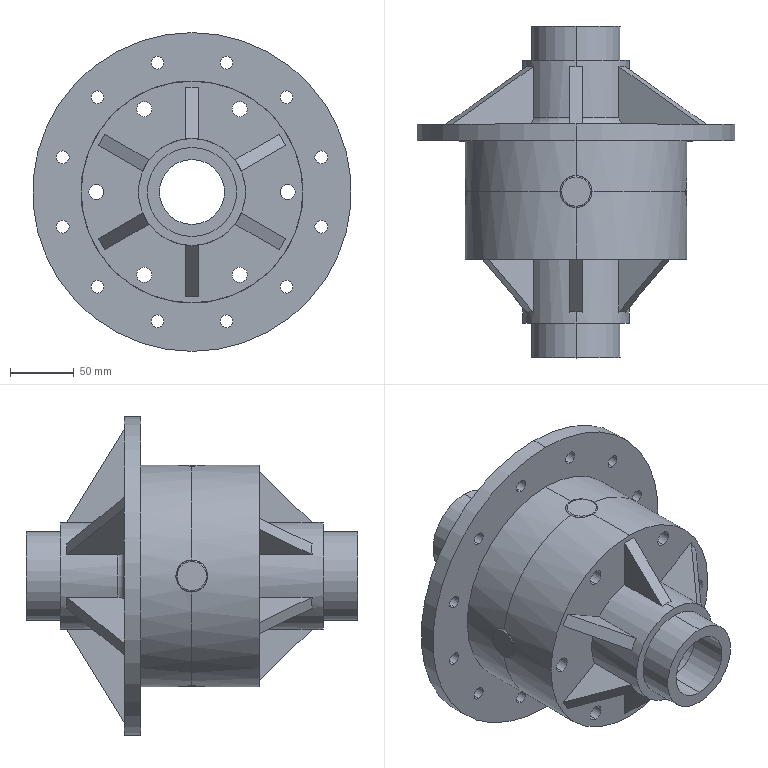Part | SolidWorks | features BaseBody 3 | 3 solids | 215 faces | box 250 x 260.308 x 250 mm | volume 2320468 mm3 | cylinder 112 | plane 65 | torus 22 | spline 16 | commonest cylinder face diameters 12 x32 10 x24 25 x16 30 x8 60 x6 51 x4